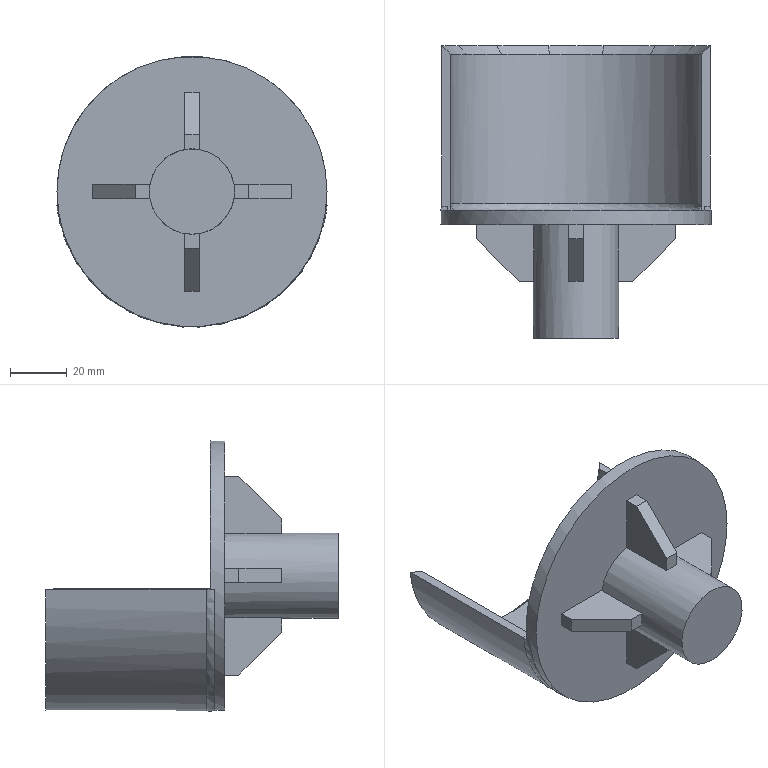Part | NX | features EXTRUDE 7, CHAMFER 5, EXTRACT_FACE 4, EXTRACT_STRING 4, Instance Feature 3, DATUM_CSYS 2, FSET 2, DIVIDE_FACE 1, FILLET_WELD 1, Pattern Feature 1, SKETCH 1, WELD_GROOVE 1 | 4 solids | 54 faces | box 95.064 x 103 x 95.3 mm | volume 92637 mm3 | plane 33 | spline 9 | cone 7 | cylinder 5 | commonest cylinder face diameters 89 x2 95 x2 30 x1